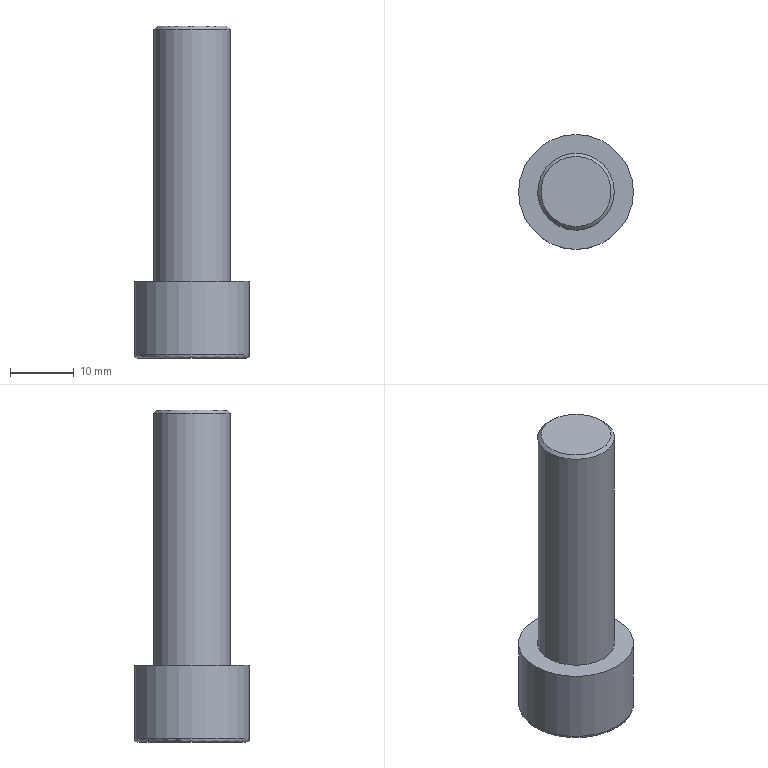Part | NX | features solid 2 | 1 solid | 14 faces | box 18 x 18 x 52 mm | volume 7050 mm3 | plane 10 | cylinder 2 | torus 1 | cone 1 | commonest cylinder face diameters 12 x1 18 x1
STEP:
#1=CARTESIAN_POINT('',(-162.113,-182.,-414.5));
#2=VERTEX_POINT('',#1);
#3=CARTESIAN_POINT('',(-159.226,-187.,-414.5));
#4=VERTEX_POINT('',#3);
#5=CARTESIAN_POINT('',(-162.113,-182.,-414.5));
#6=DIRECTION('',(0.5,-0.866,0.));
#7=VECTOR('',#6,1000.);
#8=LINE('',#5,#7);
#9=EDGE_CURVE('',#2,#4,#8,.T.);
#10=ORIENTED_EDGE('',*,*,#9,.F.);
#11=CARTESIAN_POINT('',(-167.887,-182.,-414.5));
#12=VERTEX_POINT('',#11);
#13=CARTESIAN_POINT('',(-167.887,-182.,-414.5));
#14=DIRECTION('',(1.,0.,0.));
#15=VECTOR('',#14,1000.);
#16=LINE('',#13,#15);
#17=EDGE_CURVE('',#12,#2,#16,.T.);
#18=ORIENTED_EDGE('',*,*,#17,.F.);
#19=CARTESIAN_POINT('',(-170.774,-187.,-414.5));
#20=VERTEX_POINT('',#19);
#21=CARTESIAN_POINT('',(-170.774,-187.,-414.5));
#22=DIRECTION('',(0.5,0.866,0.));
#23=VECTOR('',#22,1000.);
#24=LINE('',#21,#23);
#25=EDGE_CURVE('',#20,#12,#24,.T.);
#26=ORIENTED_EDGE('',*,*,#25,.F.);
#27=CARTESIAN_POINT('',(-167.887,-192.,-414.5));
#28=VERTEX_POINT('',#27);
#29=CARTESIAN_POINT('',(-167.887,-192.,-414.5));
#30=DIRECTION('',(-0.5,0.866,0.));
#31=VECTOR('',#30,1000.);
#32=LINE('',#29,#31);
#33=EDGE_CURVE('',#28,#20,#32,.T.);
#34=ORIENTED_EDGE('',*,*,#33,.F.);
#35=CARTESIAN_POINT('',(-162.113,-192.,-414.5));
#36=VERTEX_POINT('',#35);
#37=CARTESIAN_POINT('',(-162.113,-192.,-414.5));
#38=DIRECTION('',(-1.,0.,0.));
#39=VECTOR('',#38,1000.);
#40=LINE('',#37,#39);
#41=EDGE_CURVE('',#36,#28,#40,.T.);
#42=ORIENTED_EDGE('',*,*,#41,.F.);
#43=CARTESIAN_POINT('',(-159.226,-187.,-414.5));
#44=DIRECTION('',(-0.5,-0.866,0.));
#45=VECTOR('',#44,1000.);
#46=LINE('',#43,#45);
#47=EDGE_CURVE('',#4,#36,#46,.T.);
#48=ORIENTED_EDGE('',*,*,#47,.F.);
#49=EDGE_LOOP('',(#10,#18,#26,#34,#42,#48));
#50=FACE_BOUND('',#49,.T.);
#51=CARTESIAN_POINT('',(-165.,-178.5,-414.5));
#52=VERTEX_POINT('',#51);
#53=CARTESIAN_POINT('',(-165.,-187.,-414.5));
#54=DIRECTION('',(0.,0.,-1.));
#55=DIRECTION('',(0.,1.,0.));
#56=AXIS2_PLACEMENT_3D('',#53,#54,#55);
#57=CIRCLE('',#56,8.5);
#58=EDGE_CURVE('',#52,#52,#57,.T.);
#59=ORIENTED_EDGE('',*,*,#58,.T.);
#60=EDGE_LOOP('',(#59));
#61=FACE_BOUND('',#60,.T.);
#62=CARTESIAN_POINT('',(-165.,-187.,-414.5));
#63=DIRECTION('',(0.,0.,-1.));
#64=DIRECTION('',(0.,1.,0.));
#65=AXIS2_PLACEMENT_3D('',#62,#63,#64);
#66=PLANE('',#65);
#67=ADVANCED_FACE('',(#50,#61),#66,.T.);
#68=CARTESIAN_POINT('',(-165.,-193.,-402.5));
#69=VERTEX_POINT('',#68);
#70=CARTESIAN_POINT('',(-165.,-187.,-402.5));
#71=DIRECTION('',(0.,0.,1.));
#72=DIRECTION('',(0.,-1.,0.));
#73=AXIS2_PLACEMENT_3D('',#70,#71,#72);
#74=CIRCLE('',#73,6.);
#75=EDGE_CURVE('',#69,#69,#74,.T.);
#76=ORIENTED_EDGE('',*,*,#75,.F.);
#77=EDGE_LOOP('',(#76));
#78=FACE_BOUND('',#77,.T.);
#79=CARTESIAN_POINT('',(-156.,-187.,-402.5));
#80=VERTEX_POINT('',#79);
#81=CARTESIAN_POINT('',(-165.,-187.,-402.5));
#82=DIRECTION('',(0.,0.,-1.));
#83=DIRECTION('',(1.,0.,0.));
#84=AXIS2_PLACEMENT_3D('',#81,#82,#83);
#85=CIRCLE('',#84,9.);
#86=EDGE_CURVE('',#80,#80,#85,.T.);
#87=ORIENTED_EDGE('',*,*,#86,.F.);
#88=EDGE_LOOP('',(#87));
#89=FACE_BOUND('',#88,.T.);
#90=CARTESIAN_POINT('',(-165.,-187.,-402.5));
#91=DIRECTION('',(0.,0.,1.));
#92=DIRECTION('',(0.,-1.,0.));
#93=AXIS2_PLACEMENT_3D('',#90,#91,#92);
#94=PLANE('',#93);
#95=ADVANCED_FACE('',(#78,#89),#94,.T.);
#96=CARTESIAN_POINT('',(-165.,-178.,-414.));
#97=VERTEX_POINT('',#96);
#98=CARTESIAN_POINT('',(-165.,-187.,-414.));
#99=DIRECTION('',(0.,0.,-1.));
#100=DIRECTION('',(0.,1.,0.));
#101=AXIS2_PLACEMENT_3D('',#98,#99,#100);
#102=CIRCLE('',#101,9.);
#103=EDGE_CURVE('',#97,#97,#102,.F.);
#104=ORIENTED_EDGE('',*,*,#103,.T.);
#105=EDGE_LOOP('',(#104));
#106=FACE_BOUND('',#105,.T.);
#107=ORIENTED_EDGE('',*,*,#86,.T.);
#108=EDGE_LOOP('',(#107));
#109=FACE_BOUND('',#108,.T.);
#110=CARTESIAN_POINT('',(-165.,-187.,-402.5));
#111=DIRECTION('',(0.,0.,-1.));
#112=DIRECTION('',(1.,0.,0.));
#113=AXIS2_PLACEMENT_3D('',#110,#111,#112);
#114=CYLINDRICAL_SURFACE('',#113,9.);
#115=ADVANCED_FACE('',(#106,#109),#114,.T.);
#116=ORIENTED_EDGE('',*,*,#58,.F.);
#117=EDGE_LOOP('',(#116));
#118=FACE_BOUND('',#117,.T.);
#119=ORIENTED_EDGE('',*,*,#103,.F.);
#120=EDGE_LOOP('',(#119));
#121=FACE_BOUND('',#120,.T.);
#122=CARTESIAN_POINT('',(-165.,-187.,-414.));
#123=DIRECTION('',(0.,0.,-1.));
#124=DIRECTION('',(0.,1.,0.));
#125=AXIS2_PLACEMENT_3D('',#122,#123,#124);
#126=TOROIDAL_SURFACE('',#125,8.5,0.5);
#127=ADVANCED_FACE('',(#118,#121),#126,.T.);
#128=CARTESIAN_POINT('',(-165.,-192.5,-362.5));
#129=VERTEX_POINT('',#128);
#130=CARTESIAN_POINT('',(-165.,-187.,-362.5));
#131=DIRECTION('',(0.,0.,1.));
#132=DIRECTION('',(0.,-1.,0.));
#133=AXIS2_PLACEMENT_3D('',#130,#131,#132);
#134=CIRCLE('',#133,5.5);
#135=EDGE_CURVE('',#129,#129,#134,.T.);
#136=ORIENTED_EDGE('',*,*,#135,.T.);
#137=EDGE_LOOP('',(#136));
#138=FACE_BOUND('',#137,.T.);
#139=CARTESIAN_POINT('',(-165.,-187.,-362.5));
#140=DIRECTION('',(0.,0.,1.));
#141=DIRECTION('',(0.,-1.,0.));
#142=AXIS2_PLACEMENT_3D('',#139,#140,#141);
#143=PLANE('',#142);
#144=ADVANCED_FACE('',(#138),#143,.T.);
#145=CARTESIAN_POINT('',(-159.,-187.,-363.));
#146=VERTEX_POINT('',#145);
#147=CARTESIAN_POINT('',(-165.,-187.,-363.));
#148=DIRECTION('',(0.,0.,1.));
#149=DIRECTION('',(1.,0.,0.));
#150=AXIS2_PLACEMENT_3D('',#147,#148,#149);
#151=CIRCLE('',#150,6.);
#152=EDGE_CURVE('',#146,#146,#151,.F.);
#153=ORIENTED_EDGE('',*,*,#152,.T.);
#154=EDGE_LOOP('',(#153));
#155=FACE_BOUND('',#154,.T.);
#156=ORIENTED_EDGE('',*,*,#75,.T.);
#157=EDGE_LOOP('',(#156));
#158=FACE_BOUND('',#157,.T.);
#159=CARTESIAN_POINT('',(-165.,-187.,-362.5));
#160=DIRECTION('',(0.,0.,-1.));
#161=DIRECTION('',(1.,0.,0.));
#162=AXIS2_PLACEMENT_3D('',#159,#160,#161);
#163=CYLINDRICAL_SURFACE('',#162,6.);
#164=ADVANCED_FACE('',(#155,#158),#163,.T.);
#165=ORIENTED_EDGE('',*,*,#135,.F.);
#166=EDGE_LOOP('',(#165));
#167=FACE_BOUND('',#166,.T.);
#168=ORIENTED_EDGE('',*,*,#152,.F.);
#169=EDGE_LOOP('',(#168));
#170=FACE_BOUND('',#169,.T.);
#171=CARTESIAN_POINT('',(-165.,-187.,-363.));
#172=DIRECTION('',(0.,0.,-1.));
#173=DIRECTION('',(-1.,0.,0.));
#174=AXIS2_PLACEMENT_3D('',#171,#172,#173);
#175=CONICAL_SURFACE('',#174,6.,0.7854);
#176=ADVANCED_FACE('',(#167,#170),#175,.T.);
#177=ORIENTED_EDGE('',*,*,#9,.T.);
#178=CARTESIAN_POINT('',(-159.226,-187.,-408.5));
#179=VERTEX_POINT('',#178);
#180=CARTESIAN_POINT('',(-159.226,-187.,-408.5));
#181=DIRECTION('',(0.,0.,-1.));
#182=VECTOR('',#181,1000.);
#183=LINE('',#180,#182);
#184=EDGE_CURVE('',#179,#4,#183,.T.);
#185=ORIENTED_EDGE('',*,*,#184,.F.);
#186=CARTESIAN_POINT('',(-162.113,-182.,-408.5));
#187=VERTEX_POINT('',#186);
#188=CARTESIAN_POINT('',(-162.113,-182.,-408.5));
#189=DIRECTION('',(0.5,-0.866,0.));
#190=VECTOR('',#189,1000.);
#191=LINE('',#188,#190);
#192=EDGE_CURVE('',#187,#179,#191,.T.);
#193=ORIENTED_EDGE('',*,*,#192,.F.);
#194=CARTESIAN_POINT('',(-162.113,-182.,-408.5));
#195=DIRECTION('',(0.,0.,-1.));
#196=VECTOR('',#195,1000.);
#197=LINE('',#194,#196);
#198=EDGE_CURVE('',#187,#2,#197,.T.);
#199=ORIENTED_EDGE('',*,*,#198,.T.);
#200=EDGE_LOOP('',(#177,#185,#193,#199));
#201=FACE_BOUND('',#200,.T.);
#202=CARTESIAN_POINT('',(-160.67,-184.5,-411.5));
#203=DIRECTION('',(0.866,0.5,0.));
#204=DIRECTION('',(-0.5,0.866,0.));
#205=AXIS2_PLACEMENT_3D('',#202,#203,#204);
#206=PLANE('',#205);
#207=ADVANCED_FACE('',(#201),#206,.F.);
#208=ORIENTED_EDGE('',*,*,#17,.T.);
#209=ORIENTED_EDGE('',*,*,#198,.F.);
#210=CARTESIAN_POINT('',(-167.887,-182.,-408.5));
#211=VERTEX_POINT('',#210);
#212=CARTESIAN_POINT('',(-167.887,-182.,-408.5));
#213=DIRECTION('',(1.,0.,0.));
#214=VECTOR('',#213,1000.);
#215=LINE('',#212,#214);
#216=EDGE_CURVE('',#211,#187,#215,.T.);
#217=ORIENTED_EDGE('',*,*,#216,.F.);
#218=CARTESIAN_POINT('',(-167.887,-182.,-408.5));
#219=DIRECTION('',(0.,0.,-1.));
#220=VECTOR('',#219,1000.);
#221=LINE('',#218,#220);
#222=EDGE_CURVE('',#211,#12,#221,.T.);
#223=ORIENTED_EDGE('',*,*,#222,.T.);
#224=EDGE_LOOP('',(#208,#209,#217,#223));
#225=FACE_BOUND('',#224,.T.);
#226=CARTESIAN_POINT('',(-165.,-182.,-411.5));
#227=DIRECTION('',(0.,1.,0.));
#228=DIRECTION('',(0.,0.,1.));
#229=AXIS2_PLACEMENT_3D('',#226,#227,#228);
#230=PLANE('',#229);
#231=ADVANCED_FACE('',(#225),#230,.F.);
#232=ORIENTED_EDGE('',*,*,#25,.T.);
#233=ORIENTED_EDGE('',*,*,#222,.F.);
#234=CARTESIAN_POINT('',(-170.774,-187.,-408.5));
#235=VERTEX_POINT('',#234);
#236=CARTESIAN_POINT('',(-170.774,-187.,-408.5));
#237=DIRECTION('',(0.5,0.866,0.));
#238=VECTOR('',#237,1000.);
#239=LINE('',#236,#238);
#240=EDGE_CURVE('',#235,#211,#239,.T.);
#241=ORIENTED_EDGE('',*,*,#240,.F.);
#242=CARTESIAN_POINT('',(-170.774,-187.,-408.5));
#243=DIRECTION('',(0.,0.,-1.));
#244=VECTOR('',#243,1000.);
#245=LINE('',#242,#244);
#246=EDGE_CURVE('',#235,#20,#245,.T.);
#247=ORIENTED_EDGE('',*,*,#246,.T.);
#248=EDGE_LOOP('',(#232,#233,#241,#247));
#249=FACE_BOUND('',#248,.T.);
#250=CARTESIAN_POINT('',(-169.33,-184.5,-411.5));
#251=DIRECTION('',(-0.866,0.5,0.));
#252=DIRECTION('',(-0.5,-0.866,0.));
#253=AXIS2_PLACEMENT_3D('',#250,#251,#252);
#254=PLANE('',#253);
#255=ADVANCED_FACE('',(#249),#254,.F.);
#256=ORIENTED_EDGE('',*,*,#33,.T.);
#257=ORIENTED_EDGE('',*,*,#246,.F.);
#258=CARTESIAN_POINT('',(-167.887,-192.,-408.5));
#259=VERTEX_POINT('',#258);
#260=CARTESIAN_POINT('',(-167.887,-192.,-408.5));
#261=DIRECTION('',(-0.5,0.866,0.));
#262=VECTOR('',#261,1000.);
#263=LINE('',#260,#262);
#264=EDGE_CURVE('',#259,#235,#263,.T.);
#265=ORIENTED_EDGE('',*,*,#264,.F.);
#266=CARTESIAN_POINT('',(-167.887,-192.,-408.5));
#267=DIRECTION('',(0.,0.,-1.));
#268=VECTOR('',#267,1000.);
#269=LINE('',#266,#268);
#270=EDGE_CURVE('',#259,#28,#269,.T.);
#271=ORIENTED_EDGE('',*,*,#270,.T.);
#272=EDGE_LOOP('',(#256,#257,#265,#271));
#273=FACE_BOUND('',#272,.T.);
#274=CARTESIAN_POINT('',(-169.33,-189.5,-411.5));
#275=DIRECTION('',(-0.866,-0.5,0.));
#276=DIRECTION('',(0.5,-0.866,0.));
#277=AXIS2_PLACEMENT_3D('',#274,#275,#276);
#278=PLANE('',#277);
#279=ADVANCED_FACE('',(#273),#278,.F.);
#280=ORIENTED_EDGE('',*,*,#41,.T.);
#281=ORIENTED_EDGE('',*,*,#270,.F.);
#282=CARTESIAN_POINT('',(-162.113,-192.,-408.5));
#283=VERTEX_POINT('',#282);
#284=CARTESIAN_POINT('',(-162.113,-192.,-408.5));
#285=DIRECTION('',(-1.,0.,0.));
#286=VECTOR('',#285,1000.);
#287=LINE('',#284,#286);
#288=EDGE_CURVE('',#283,#259,#287,.T.);
#289=ORIENTED_EDGE('',*,*,#288,.F.);
#290=CARTESIAN_POINT('',(-162.113,-192.,-408.5));
#291=DIRECTION('',(0.,0.,-1.));
#292=VECTOR('',#291,1000.);
#293=LINE('',#290,#292);
#294=EDGE_CURVE('',#283,#36,#293,.T.);
#295=ORIENTED_EDGE('',*,*,#294,.T.);
#296=EDGE_LOOP('',(#280,#281,#289,#295));
#297=FACE_BOUND('',#296,.T.);
#298=CARTESIAN_POINT('',(-165.,-192.,-411.5));
#299=DIRECTION('',(0.,-1.,0.));
#300=DIRECTION('',(0.,0.,-1.));
#301=AXIS2_PLACEMENT_3D('',#298,#299,#300);
#302=PLANE('',#301);
#303=ADVANCED_FACE('',(#297),#302,.F.);
#304=ORIENTED_EDGE('',*,*,#47,.T.);
#305=ORIENTED_EDGE('',*,*,#294,.F.);
#306=CARTESIAN_POINT('',(-159.226,-187.,-408.5));
#307=DIRECTION('',(-0.5,-0.866,0.));
#308=VECTOR('',#307,1000.);
#309=LINE('',#306,#308);
#310=EDGE_CURVE('',#179,#283,#309,.T.);
#311=ORIENTED_EDGE('',*,*,#310,.F.);
#312=ORIENTED_EDGE('',*,*,#184,.T.);
#313=EDGE_LOOP('',(#304,#305,#311,#312));
#314=FACE_BOUND('',#313,.T.);
#315=CARTESIAN_POINT('',(-160.67,-189.5,-411.5));
#316=DIRECTION('',(0.866,-0.5,0.));
#317=DIRECTION('',(0.5,0.866,0.));
#318=AXIS2_PLACEMENT_3D('',#315,#316,#317);
#319=PLANE('',#318);
#320=ADVANCED_FACE('',(#314),#319,.F.);
#321=ORIENTED_EDGE('',*,*,#310,.T.);
#322=ORIENTED_EDGE('',*,*,#288,.T.);
#323=ORIENTED_EDGE('',*,*,#264,.T.);
#324=ORIENTED_EDGE('',*,*,#240,.T.);
#325=ORIENTED_EDGE('',*,*,#216,.T.);
#326=ORIENTED_EDGE('',*,*,#192,.T.);
#327=EDGE_LOOP('',(#321,#322,#323,#324,#325,#326));
#328=FACE_BOUND('',#327,.T.);
#329=CARTESIAN_POINT('',(-165.,-187.,-408.5));
#330=DIRECTION('',(0.,0.,1.));
#331=DIRECTION('',(0.,-1.,0.));
#332=AXIS2_PLACEMENT_3D('',#329,#330,#331);
#333=PLANE('',#332);
#334=ADVANCED_FACE('',(#328),#333,.F.);
#335=CLOSED_SHELL('',(#67,#95,#115,#127,#144,#164,#176,#207,#231,#255,#279,#303,#320,#334));
#336=MANIFOLD_SOLID_BREP('',#335);
#337=(LENGTH_UNIT()NAMED_UNIT(*)SI_UNIT(.MILLI.,.METRE.));
#338=UNCERTAINTY_MEASURE_WITH_UNIT(LENGTH_MEASURE(0.00001),#337,'','');
#339=(NAMED_UNIT(*)PLANE_ANGLE_UNIT()SI_UNIT($,.RADIAN.));
#340=(NAMED_UNIT(*)SI_UNIT($,.STERADIAN.)SOLID_ANGLE_UNIT());
#341=(GEOMETRIC_REPRESENTATION_CONTEXT(3)GLOBAL_UNCERTAINTY_ASSIGNED_CONTEXT((#338))GLOBAL_UNIT_ASSIGNED_CONTEXT((#337,#339,#340))REPRESENTATION_CONTEXT('',''));
#342=ADVANCED_BREP_SHAPE_REPRESENTATION('',(#336),#341);